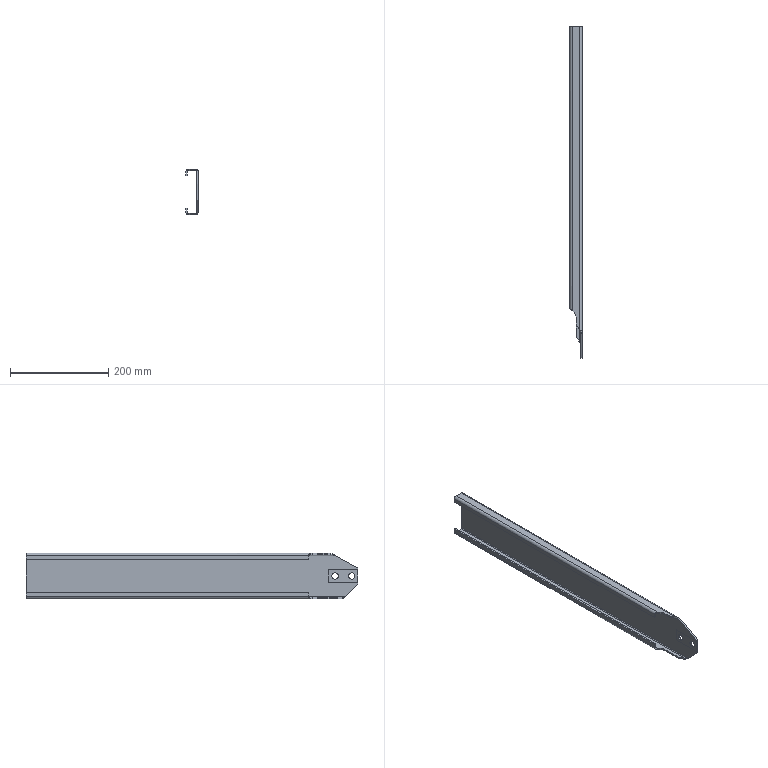Part | SolidWorks | features ICE 4, FlatPattern 1, SMBaseFlange 1, SheetMetal 1 | 1 solid | 56 faces | box 24.9 x 675 x 92.9 mm | volume 303030 mm3 | plane 36 | cylinder 14 | spline 6 | commonest cylinder face diameters 4 x4 10.4 x4 13 x4 50 x2